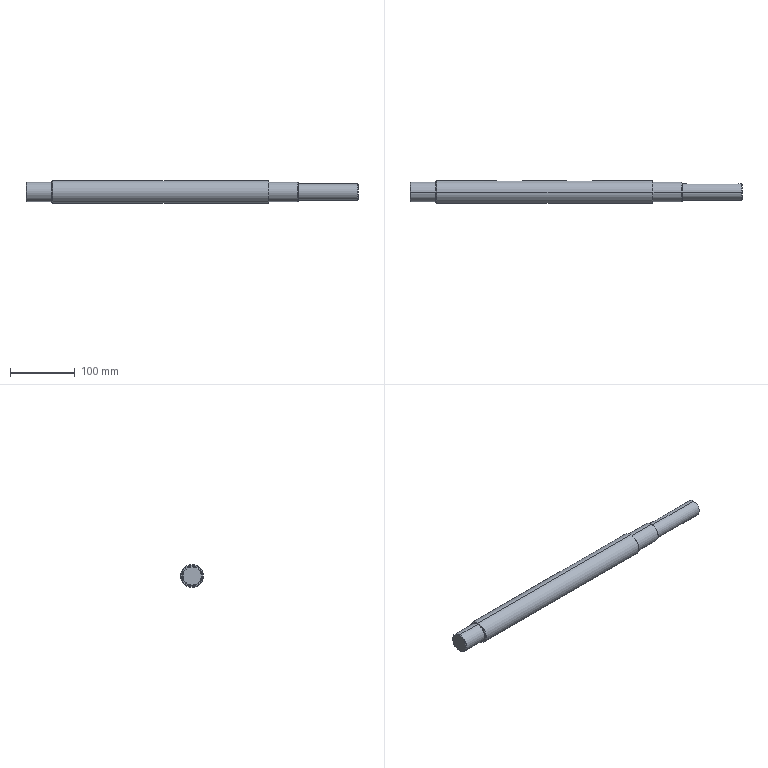Part | SolidWorks | features ICE 2, Chamfer 1, HoleWzd 1, Revolution 1 | 1 solid | 46 faces | box 511 x 35 x 35 mm | volume 419085 mm3 | cylinder 18 | cone 14 | plane 14 | commonest cylinder face diameters 5 x4 10 x4 30 x4 8 x2 25 x2 35 x2
STEP:
#1=CARTESIAN_POINT('',(284.,0.,-3.5));
#2=VERTEX_POINT('',#1);
#3=CARTESIAN_POINT('',(284.,0.,-8.5));
#4=VERTEX_POINT('',#3);
#5=CARTESIAN_POINT('',(284.,0.,-6.));
#6=DIRECTION('',(1.,0.,0.));
#7=DIRECTION('',(0.,0.,-1.));
#8=AXIS2_PLACEMENT_3D('',#5,#6,#7);
#9=CIRCLE('',#8,2.5);
#10=EDGE_CURVE('',#2,#4,#9,.T.);
#11=ORIENTED_EDGE('',*,*,#10,.F.);
#12=CARTESIAN_POINT('',(304.,0.,-3.5));
#13=VERTEX_POINT('',#12);
#14=CARTESIAN_POINT('',(304.,0.,-3.5));
#15=DIRECTION('',(1.,0.,0.));
#16=VECTOR('',#15,1000.);
#17=LINE('',#14,#16);
#18=EDGE_CURVE('',#2,#13,#17,.T.);
#19=ORIENTED_EDGE('',*,*,#18,.T.);
#20=CARTESIAN_POINT('',(304.,0.,-8.5));
#21=VERTEX_POINT('',#20);
#22=CARTESIAN_POINT('',(304.,0.,-6.));
#23=DIRECTION('',(1.,0.,0.));
#24=DIRECTION('',(0.,0.,-1.));
#25=AXIS2_PLACEMENT_3D('',#22,#23,#24);
#26=CIRCLE('',#25,2.5);
#27=EDGE_CURVE('',#13,#21,#26,.T.);
#28=ORIENTED_EDGE('',*,*,#27,.T.);
#29=CARTESIAN_POINT('',(304.,0.,-8.5));
#30=DIRECTION('',(1.,0.,0.));
#31=VECTOR('',#30,1000.);
#32=LINE('',#29,#31);
#33=EDGE_CURVE('',#4,#21,#32,.T.);
#34=ORIENTED_EDGE('',*,*,#33,.F.);
#35=EDGE_LOOP('',(#11,#19,#28,#34));
#36=FACE_OUTER_BOUND('',#35,.T.);
#37=CARTESIAN_POINT('',(304.,0.,-6.));
#38=DIRECTION('',(1.,0.,0.));
#39=DIRECTION('',(0.,0.,-1.));
#40=AXIS2_PLACEMENT_3D('',#37,#38,#39);
#41=CYLINDRICAL_SURFACE('',#40,2.5);
#42=ADVANCED_FACE('',(#36),#41,.F.);
#43=CARTESIAN_POINT('',(282.498,0.,-6.));
#44=VERTEX_POINT('',#43);
#45=CARTESIAN_POINT('',(284.,0.,-8.5));
#46=DIRECTION('',(0.515,0.,-0.8572));
#47=VECTOR('',#46,1000.);
#48=LINE('',#45,#47);
#49=EDGE_CURVE('',#44,#4,#48,.T.);
#50=ORIENTED_EDGE('',*,*,#49,.F.);
#51=CARTESIAN_POINT('',(284.,0.,-3.5));
#52=DIRECTION('',(0.515,0.,0.8572));
#53=VECTOR('',#52,1000.);
#54=LINE('',#51,#53);
#55=EDGE_CURVE('',#44,#2,#54,.T.);
#56=ORIENTED_EDGE('',*,*,#55,.T.);
#57=ORIENTED_EDGE('',*,*,#10,.T.);
#58=EDGE_LOOP('',(#50,#56,#57));
#59=FACE_OUTER_BOUND('',#58,.T.);
#60=CARTESIAN_POINT('',(284.,0.,-6.));
#61=DIRECTION('',(1.,0.,0.));
#62=DIRECTION('',(0.,0.,-1.));
#63=AXIS2_PLACEMENT_3D('',#60,#61,#62);
#64=CONICAL_SURFACE('',#63,2.5,1.03);
#65=ADVANCED_FACE('',(#59),#64,.F.);
#66=CARTESIAN_POINT('',(284.,0.,8.5));
#67=VERTEX_POINT('',#66);
#68=CARTESIAN_POINT('',(284.,0.,3.5));
#69=VERTEX_POINT('',#68);
#70=CARTESIAN_POINT('',(284.,0.,6.));
#71=DIRECTION('',(1.,0.,0.));
#72=DIRECTION('',(0.,0.,-1.));
#73=AXIS2_PLACEMENT_3D('',#70,#71,#72);
#74=CIRCLE('',#73,2.5);
#75=EDGE_CURVE('',#67,#69,#74,.T.);
#76=ORIENTED_EDGE('',*,*,#75,.F.);
#77=CARTESIAN_POINT('',(304.,0.,8.5));
#78=VERTEX_POINT('',#77);
#79=CARTESIAN_POINT('',(304.,0.,8.5));
#80=DIRECTION('',(1.,0.,0.));
#81=VECTOR('',#80,1000.);
#82=LINE('',#79,#81);
#83=EDGE_CURVE('',#67,#78,#82,.T.);
#84=ORIENTED_EDGE('',*,*,#83,.T.);
#85=CARTESIAN_POINT('',(304.,0.,3.5));
#86=VERTEX_POINT('',#85);
#87=CARTESIAN_POINT('',(304.,0.,6.));
#88=DIRECTION('',(1.,0.,0.));
#89=DIRECTION('',(0.,0.,-1.));
#90=AXIS2_PLACEMENT_3D('',#87,#88,#89);
#91=CIRCLE('',#90,2.5);
#92=EDGE_CURVE('',#78,#86,#91,.T.);
#93=ORIENTED_EDGE('',*,*,#92,.T.);
#94=CARTESIAN_POINT('',(304.,0.,3.5));
#95=DIRECTION('',(1.,0.,0.));
#96=VECTOR('',#95,1000.);
#97=LINE('',#94,#96);
#98=EDGE_CURVE('',#69,#86,#97,.T.);
#99=ORIENTED_EDGE('',*,*,#98,.F.);
#100=EDGE_LOOP('',(#76,#84,#93,#99));
#101=FACE_OUTER_BOUND('',#100,.T.);
#102=CARTESIAN_POINT('',(304.,0.,6.));
#103=DIRECTION('',(1.,0.,0.));
#104=DIRECTION('',(0.,0.,-1.));
#105=AXIS2_PLACEMENT_3D('',#102,#103,#104);
#106=CYLINDRICAL_SURFACE('',#105,2.5);
#107=ADVANCED_FACE('',(#101),#106,.F.);
#108=CARTESIAN_POINT('',(282.498,0.,6.));
#109=VERTEX_POINT('',#108);
#110=CARTESIAN_POINT('',(284.,0.,3.5));
#111=DIRECTION('',(0.515,0.,-0.8572));
#112=VECTOR('',#111,1000.);
#113=LINE('',#110,#112);
#114=EDGE_CURVE('',#109,#69,#113,.T.);
#115=ORIENTED_EDGE('',*,*,#114,.F.);
#116=CARTESIAN_POINT('',(284.,0.,8.5));
#117=DIRECTION('',(0.515,0.,0.8572));
#118=VECTOR('',#117,1000.);
#119=LINE('',#116,#118);
#120=EDGE_CURVE('',#109,#67,#119,.T.);
#121=ORIENTED_EDGE('',*,*,#120,.T.);
#122=ORIENTED_EDGE('',*,*,#75,.T.);
#123=EDGE_LOOP('',(#115,#121,#122));
#124=FACE_OUTER_BOUND('',#123,.T.);
#125=CARTESIAN_POINT('',(284.,0.,6.));
#126=DIRECTION('',(1.,0.,0.));
#127=DIRECTION('',(0.,0.,-1.));
#128=AXIS2_PLACEMENT_3D('',#125,#126,#127);
#129=CONICAL_SURFACE('',#128,2.5,1.03);
#130=ADVANCED_FACE('',(#124),#129,.F.);
#131=CARTESIAN_POINT('',(-207.,0.,14.));
#132=VERTEX_POINT('',#131);
#133=CARTESIAN_POINT('',(-207.,0.,-14.));
#134=VERTEX_POINT('',#133);
#135=CARTESIAN_POINT('',(-207.,0.,0.));
#136=DIRECTION('',(-1.,0.,0.));
#137=DIRECTION('',(0.,0.,1.));
#138=AXIS2_PLACEMENT_3D('',#135,#136,#137);
#139=CIRCLE('',#138,14.);
#140=EDGE_CURVE('',#132,#134,#139,.T.);
#141=ORIENTED_EDGE('',*,*,#140,.F.);
#142=CARTESIAN_POINT('',(-206.,0.,15.));
#143=VERTEX_POINT('',#142);
#144=CARTESIAN_POINT('',(-206.,0.,15.));
#145=DIRECTION('',(0.7071,0.,0.7071));
#146=VECTOR('',#145,1000.);
#147=LINE('',#144,#146);
#148=EDGE_CURVE('',#132,#143,#147,.T.);
#149=ORIENTED_EDGE('',*,*,#148,.T.);
#150=CARTESIAN_POINT('',(-206.,0.,-15.));
#151=VERTEX_POINT('',#150);
#152=CARTESIAN_POINT('',(-206.,0.,0.));
#153=DIRECTION('',(1.,0.,0.));
#154=DIRECTION('',(0.,0.,1.));
#155=AXIS2_PLACEMENT_3D('',#152,#153,#154);
#156=CIRCLE('',#155,15.);
#157=EDGE_CURVE('',#151,#143,#156,.T.);
#158=ORIENTED_EDGE('',*,*,#157,.F.);
#159=CARTESIAN_POINT('',(-206.,0.,-15.));
#160=DIRECTION('',(0.7071,0.,-0.7071));
#161=VECTOR('',#160,1000.);
#162=LINE('',#159,#161);
#163=EDGE_CURVE('',#134,#151,#162,.T.);
#164=ORIENTED_EDGE('',*,*,#163,.F.);
#165=EDGE_LOOP('',(#141,#149,#158,#164));
#166=FACE_OUTER_BOUND('',#165,.T.);
#167=CARTESIAN_POINT('',(-206.,0.,0.));
#168=DIRECTION('',(1.,0.,0.));
#169=DIRECTION('',(0.,0.,-1.));
#170=AXIS2_PLACEMENT_3D('',#167,#168,#169);
#171=CONICAL_SURFACE('',#170,15.,0.7854);
#172=ADVANCED_FACE('',(#166),#171,.T.);
#173=CARTESIAN_POINT('',(167.,0.,-16.5));
#174=VERTEX_POINT('',#173);
#175=CARTESIAN_POINT('',(167.,0.,16.5));
#176=VERTEX_POINT('',#175);
#177=CARTESIAN_POINT('',(167.,0.,0.));
#178=DIRECTION('',(1.,0.,0.));
#179=DIRECTION('',(0.,0.,-1.));
#180=AXIS2_PLACEMENT_3D('',#177,#178,#179);
#181=CIRCLE('',#180,16.5);
#182=EDGE_CURVE('',#174,#176,#181,.T.);
#183=ORIENTED_EDGE('',*,*,#182,.F.);
#184=CARTESIAN_POINT('',(166.,0.,-17.5));
#185=VERTEX_POINT('',#184);
#186=CARTESIAN_POINT('',(167.,0.,-16.5));
#187=DIRECTION('',(-0.7071,0.,-0.7071));
#188=VECTOR('',#187,1000.);
#189=LINE('',#186,#188);
#190=EDGE_CURVE('',#174,#185,#189,.T.);
#191=ORIENTED_EDGE('',*,*,#190,.T.);
#192=CARTESIAN_POINT('',(166.,0.,17.5));
#193=VERTEX_POINT('',#192);
#194=CARTESIAN_POINT('',(166.,0.,0.));
#195=DIRECTION('',(-1.,0.,0.));
#196=DIRECTION('',(0.,0.,-1.));
#197=AXIS2_PLACEMENT_3D('',#194,#195,#196);
#198=CIRCLE('',#197,17.5);
#199=EDGE_CURVE('',#193,#185,#198,.T.);
#200=ORIENTED_EDGE('',*,*,#199,.F.);
#201=CARTESIAN_POINT('',(167.,0.,16.5));
#202=DIRECTION('',(-0.7071,0.,0.7071));
#203=VECTOR('',#202,1000.);
#204=LINE('',#201,#203);
#205=EDGE_CURVE('',#176,#193,#204,.T.);
#206=ORIENTED_EDGE('',*,*,#205,.F.);
#207=EDGE_LOOP('',(#183,#191,#200,#206));
#208=FACE_OUTER_BOUND('',#207,.T.);
#209=CARTESIAN_POINT('',(167.,0.,0.));
#210=DIRECTION('',(-1.,0.,0.));
#211=DIRECTION('',(0.,0.,1.));
#212=AXIS2_PLACEMENT_3D('',#209,#210,#211);
#213=CONICAL_SURFACE('',#212,16.5,0.7854);
#214=ADVANCED_FACE('',(#208),#213,.T.);
#215=CARTESIAN_POINT('',(212.,0.,-14.));
#216=VERTEX_POINT('',#215);
#217=CARTESIAN_POINT('',(212.,0.,14.));
#218=VERTEX_POINT('',#217);
#219=CARTESIAN_POINT('',(212.,0.,0.));
#220=DIRECTION('',(1.,0.,0.));
#221=DIRECTION('',(0.,0.,-1.));
#222=AXIS2_PLACEMENT_3D('',#219,#220,#221);
#223=CIRCLE('',#222,14.);
#224=EDGE_CURVE('',#216,#218,#223,.T.);
#225=ORIENTED_EDGE('',*,*,#224,.F.);
#226=CARTESIAN_POINT('',(211.,0.,-15.));
#227=VERTEX_POINT('',#226);
#228=CARTESIAN_POINT('',(212.,0.,-14.));
#229=DIRECTION('',(-0.7071,0.,-0.7071));
#230=VECTOR('',#229,1000.);
#231=LINE('',#228,#230);
#232=EDGE_CURVE('',#216,#227,#231,.T.);
#233=ORIENTED_EDGE('',*,*,#232,.T.);
#234=CARTESIAN_POINT('',(211.,0.,15.));
#235=VERTEX_POINT('',#234);
#236=CARTESIAN_POINT('',(211.,0.,0.));
#237=DIRECTION('',(-1.,0.,0.));
#238=DIRECTION('',(0.,0.,-1.));
#239=AXIS2_PLACEMENT_3D('',#236,#237,#238);
#240=CIRCLE('',#239,15.);
#241=EDGE_CURVE('',#235,#227,#240,.T.);
#242=ORIENTED_EDGE('',*,*,#241,.F.);
#243=CARTESIAN_POINT('',(212.,0.,14.));
#244=DIRECTION('',(-0.7071,0.,0.7071));
#245=VECTOR('',#244,1000.);
#246=LINE('',#243,#245);
#247=EDGE_CURVE('',#218,#235,#246,.T.);
#248=ORIENTED_EDGE('',*,*,#247,.F.);
#249=EDGE_LOOP('',(#225,#233,#242,#248));
#250=FACE_OUTER_BOUND('',#249,.T.);
#251=CARTESIAN_POINT('',(212.,0.,0.));
#252=DIRECTION('',(-1.,0.,0.));
#253=DIRECTION('',(0.,0.,1.));
#254=AXIS2_PLACEMENT_3D('',#251,#252,#253);
#255=CONICAL_SURFACE('',#254,14.,0.7854);
#256=ADVANCED_FACE('',(#250),#255,.T.);
#257=CARTESIAN_POINT('',(304.,0.,-11.5));
#258=VERTEX_POINT('',#257);
#259=CARTESIAN_POINT('',(304.,0.,11.5));
#260=VERTEX_POINT('',#259);
#261=CARTESIAN_POINT('',(304.,0.,0.));
#262=DIRECTION('',(1.,0.,0.));
#263=DIRECTION('',(0.,0.,-1.));
#264=AXIS2_PLACEMENT_3D('',#261,#262,#263);
#265=CIRCLE('',#264,11.5);
#266=EDGE_CURVE('',#258,#260,#265,.T.);
#267=ORIENTED_EDGE('',*,*,#266,.F.);
#268=CARTESIAN_POINT('',(303.,0.,-12.5));
#269=VERTEX_POINT('',#268);
#270=CARTESIAN_POINT('',(304.,0.,-11.5));
#271=DIRECTION('',(-0.7071,0.,-0.7071));
#272=VECTOR('',#271,1000.);
#273=LINE('',#270,#272);
#274=EDGE_CURVE('',#258,#269,#273,.T.);
#275=ORIENTED_EDGE('',*,*,#274,.T.);
#276=CARTESIAN_POINT('',(303.,0.,12.5));
#277=VERTEX_POINT('',#276);
#278=CARTESIAN_POINT('',(303.,0.,0.));
#279=DIRECTION('',(-1.,0.,0.));
#280=DIRECTION('',(0.,0.,-1.));
#281=AXIS2_PLACEMENT_3D('',#278,#279,#280);
#282=CIRCLE('',#281,12.5);
#283=EDGE_CURVE('',#277,#269,#282,.T.);
#284=ORIENTED_EDGE('',*,*,#283,.F.);
#285=CARTESIAN_POINT('',(304.,0.,11.5));
#286=DIRECTION('',(-0.7071,0.,0.7071));
#287=VECTOR('',#286,1000.);
#288=LINE('',#285,#287);
#289=EDGE_CURVE('',#260,#277,#288,.T.);
#290=ORIENTED_EDGE('',*,*,#289,.F.);
#291=EDGE_LOOP('',(#267,#275,#284,#290));
#292=FACE_OUTER_BOUND('',#291,.T.);
#293=CARTESIAN_POINT('',(304.,0.,0.));
#294=DIRECTION('',(-1.,0.,0.));
#295=DIRECTION('',(0.,0.,1.));
#296=AXIS2_PLACEMENT_3D('',#293,#294,#295);
#297=CONICAL_SURFACE('',#296,11.5,0.7854);
#298=ADVANCED_FACE('',(#292),#297,.T.);
#299=CARTESIAN_POINT('',(-167.,0.,16.5));
#300=VERTEX_POINT('',#299);
#301=CARTESIAN_POINT('',(-167.,0.,-16.5));
#302=VERTEX_POINT('',#301);
#303=CARTESIAN_POINT('',(-167.,0.,0.));
#304=DIRECTION('',(-1.,0.,0.));
#305=DIRECTION('',(0.,0.,1.));
#306=AXIS2_PLACEMENT_3D('',#303,#304,#305);
#307=CIRCLE('',#306,16.5);
#308=EDGE_CURVE('',#300,#302,#307,.T.);
#309=ORIENTED_EDGE('',*,*,#308,.F.);
#310=CARTESIAN_POINT('',(-166.,0.,17.5));
#311=VERTEX_POINT('',#310);
#312=CARTESIAN_POINT('',(-166.,0.,17.5));
#313=DIRECTION('',(0.7071,0.,0.7071));
#314=VECTOR('',#313,1000.);
#315=LINE('',#312,#314);
#316=EDGE_CURVE('',#300,#311,#315,.T.);
#317=ORIENTED_EDGE('',*,*,#316,.T.);
#318=CARTESIAN_POINT('',(-166.,0.,-17.5));
#319=VERTEX_POINT('',#318);
#320=CARTESIAN_POINT('',(-166.,0.,0.));
#321=DIRECTION('',(1.,0.,0.));
#322=DIRECTION('',(0.,0.,1.));
#323=AXIS2_PLACEMENT_3D('',#320,#321,#322);
#324=CIRCLE('',#323,17.5);
#325=EDGE_CURVE('',#319,#311,#324,.T.);
#326=ORIENTED_EDGE('',*,*,#325,.F.);
#327=CARTESIAN_POINT('',(-166.,0.,-17.5));
#328=DIRECTION('',(0.7071,0.,-0.7071));
#329=VECTOR('',#328,1000.);
#330=LINE('',#327,#329);
#331=EDGE_CURVE('',#302,#319,#330,.T.);
#332=ORIENTED_EDGE('',*,*,#331,.F.);
#333=EDGE_LOOP('',(#309,#317,#326,#332));
#334=FACE_OUTER_BOUND('',#333,.T.);
#335=CARTESIAN_POINT('',(-166.,0.,0.));
#336=DIRECTION('',(1.,0.,0.));
#337=DIRECTION('',(0.,0.,-1.));
#338=AXIS2_PLACEMENT_3D('',#335,#336,#337);
#339=CONICAL_SURFACE('',#338,17.5,0.7854);
#340=ADVANCED_FACE('',(#334),#339,.T.);
#341=CARTESIAN_POINT('',(167.,0.,-15.));
#342=VERTEX_POINT('',#341);
#343=CARTESIAN_POINT('',(167.,0.,15.));
#344=VERTEX_POINT('',#343);
#345=CARTESIAN_POINT('',(167.,0.,0.));
#346=DIRECTION('',(1.,0.,0.));
#347=DIRECTION('',(0.,0.,-1.));
#348=AXIS2_PLACEMENT_3D('',#345,#346,#347);
#349=CIRCLE('',#348,15.);
#350=EDGE_CURVE('',#342,#344,#349,.T.);
#351=ORIENTED_EDGE('',*,*,#350,.T.);
#352=CARTESIAN_POINT('',(0.,0.,15.));
#353=DIRECTION('',(1.,0.,0.));
#354=VECTOR('',#353,1000.);
#355=LINE('',#352,#354);
#356=EDGE_CURVE('',#344,#235,#355,.T.);
#357=ORIENTED_EDGE('',*,*,#356,.T.);
#358=ORIENTED_EDGE('',*,*,#241,.T.);
#359=CARTESIAN_POINT('',(0.,0.,-15.));
#360=DIRECTION('',(1.,0.,0.));
#361=VECTOR('',#360,1000.);
#362=LINE('',#359,#361);
#363=EDGE_CURVE('',#342,#227,#362,.T.);
#364=ORIENTED_EDGE('',*,*,#363,.F.);
#365=EDGE_LOOP('',(#351,#357,#358,#364));
#366=FACE_OUTER_BOUND('',#365,.T.);
#367=CARTESIAN_POINT('',(0.,0.,0.));
#368=DIRECTION('',(1.,0.,0.));
#369=DIRECTION('',(0.,0.,-1.));
#370=AXIS2_PLACEMENT_3D('',#367,#368,#369);
#371=CYLINDRICAL_SURFACE('',#370,15.);
#372=ADVANCED_FACE('',(#366),#371,.T.);
#373=CARTESIAN_POINT('',(295.,11.843,4.));
#374=VERTEX_POINT('',#373);
#375=CARTESIAN_POINT('',(295.,11.843,-4.));
#376=VERTEX_POINT('',#375);
#377=CARTESIAN_POINT('',(295.,11.843,4.));
#378=CARTESIAN_POINT('',(295.266,11.843,4.));
#379=CARTESIAN_POINT('',(295.527,11.852,3.974));
#380=CARTESIAN_POINT('',(296.041,11.886,3.871));
#381=CARTESIAN_POINT('',(296.296,11.911,3.793));
#382=CARTESIAN_POINT('',(296.779,11.973,3.592));
#383=CARTESIAN_POINT('',(297.008,12.01,3.469));
#384=CARTESIAN_POINT('',(297.441,12.09,3.179));
#385=CARTESIAN_POINT('',(297.645,12.133,3.012));
#386=CARTESIAN_POINT('',(298.011,12.218,2.646));
#387=CARTESIAN_POINT('',(298.176,12.26,2.445));
#388=CARTESIAN_POINT('',(298.469,12.34,2.009));
#389=CARTESIAN_POINT('',(298.592,12.375,1.779));
#390=CARTESIAN_POINT('',(298.792,12.435,1.299));
#391=CARTESIAN_POINT('',(298.87,12.459,1.045));
#392=CARTESIAN_POINT('',(298.974,12.492,0.5276));
#393=CARTESIAN_POINT('',(299.,12.5,0.2669));
#394=CARTESIAN_POINT('',(299.,12.5,-0.2587));
#395=CARTESIAN_POINT('',(298.974,12.492,-0.5256));
#396=CARTESIAN_POINT('',(298.871,12.459,-1.04));
#397=CARTESIAN_POINT('',(298.795,12.436,-1.29));
#398=CARTESIAN_POINT('',(298.593,12.375,-1.777));
#399=CARTESIAN_POINT('',(298.469,12.34,-2.008));
#400=CARTESIAN_POINT('',(298.18,12.262,-2.44));
#401=CARTESIAN_POINT('',(298.013,12.219,-2.643));
#402=CARTESIAN_POINT('',(297.645,12.133,-3.012));
#403=CARTESIAN_POINT('',(297.445,12.091,-3.176));
#404=CARTESIAN_POINT('',(297.013,12.011,-3.466));
#405=CARTESIAN_POINT('',(296.78,11.973,-3.592));
#406=CARTESIAN_POINT('',(296.298,11.911,-3.792));
#407=CARTESIAN_POINT('',(296.049,11.886,-3.869));
#408=CARTESIAN_POINT('',(295.532,11.852,-3.973));
#409=CARTESIAN_POINT('',(295.266,11.843,-4.));
#410=CARTESIAN_POINT('',(295.,11.843,-4.));
#411=B_SPLINE_CURVE_WITH_KNOTS('',3,(#377,#378,#379,#380,#381,#382,#383,#384,#385,#386,#387,#388,#389,#390,#391,#392,#393,#394,#395,#396,#397,#398,#399,#400,#401,#402,#403,#404,#405,#406,#407,#408,#409,#410),.UNSPECIFIED.,.F.,.F.,(4,2,2,2,2,2,2,2,2,2,2,2,2,2,2,2,4),(0.,0.0007865,0.001573,0.00236,0.003146,0.003933,0.004719,0.005506,0.006292,0.007079,0.007865,0.008652,0.009438,0.01022,0.01101,0.0118,0.01258),.UNSPECIFIED.);
#412=EDGE_CURVE('',#374,#376,#411,.T.);
#413=ORIENTED_EDGE('',*,*,#412,.F.);
#414=CARTESIAN_POINT('',(223.,11.843,4.));
#415=VERTEX_POINT('',#414);
#416=CARTESIAN_POINT('',(0.,11.843,4.));
#417=DIRECTION('',(1.,0.,0.));
#418=VECTOR('',#417,1000.);
#419=LINE('',#416,#418);
#420=EDGE_CURVE('',#415,#374,#419,.T.);
#421=ORIENTED_EDGE('',*,*,#420,.F.);
#422=CARTESIAN_POINT('',(223.,11.843,-4.));
#423=VERTEX_POINT('',#422);
#424=CARTESIAN_POINT('',(223.,11.843,-4.));
#425=CARTESIAN_POINT('',(222.734,11.843,-4.));
#426=CARTESIAN_POINT('',(222.473,11.852,-3.974));
#427=CARTESIAN_POINT('',(221.959,11.886,-3.871));
#428=CARTESIAN_POINT('',(221.704,11.911,-3.793));
#429=CARTESIAN_POINT('',(221.221,11.973,-3.592));
#430=CARTESIAN_POINT('',(220.992,12.01,-3.469));
#431=CARTESIAN_POINT('',(220.559,12.09,-3.179));
#432=CARTESIAN_POINT('',(220.355,12.133,-3.012));
#433=CARTESIAN_POINT('',(219.989,12.218,-2.646));
#434=CARTESIAN_POINT('',(219.824,12.26,-2.445));
#435=CARTESIAN_POINT('',(219.531,12.34,-2.009));
#436=CARTESIAN_POINT('',(219.408,12.375,-1.779));
#437=CARTESIAN_POINT('',(219.208,12.435,-1.299));
#438=CARTESIAN_POINT('',(219.13,12.459,-1.045));
#439=CARTESIAN_POINT('',(219.026,12.492,-0.5276));
#440=CARTESIAN_POINT('',(219.,12.5,-0.2669));
#441=CARTESIAN_POINT('',(219.,12.5,0.2587));
#442=CARTESIAN_POINT('',(219.026,12.492,0.5256));
#443=CARTESIAN_POINT('',(219.129,12.459,1.04));
#444=CARTESIAN_POINT('',(219.205,12.436,1.29));
#445=CARTESIAN_POINT('',(219.407,12.375,1.777));
#446=CARTESIAN_POINT('',(219.531,12.34,2.008));
#447=CARTESIAN_POINT('',(219.82,12.262,2.44));
#448=CARTESIAN_POINT('',(219.987,12.219,2.643));
#449=CARTESIAN_POINT('',(220.355,12.133,3.012));
#450=CARTESIAN_POINT('',(220.555,12.091,3.176));
#451=CARTESIAN_POINT('',(220.987,12.011,3.466));
#452=CARTESIAN_POINT('',(221.22,11.973,3.592));
#453=CARTESIAN_POINT('',(221.702,11.911,3.792));
#454=CARTESIAN_POINT('',(221.951,11.886,3.869));
#455=CARTESIAN_POINT('',(222.468,11.852,3.973));
#456=CARTESIAN_POINT('',(222.734,11.843,4.));
#457=CARTESIAN_POINT('',(223.,11.843,4.));
#458=B_SPLINE_CURVE_WITH_KNOTS('',3,(#424,#425,#426,#427,#428,#429,#430,#431,#432,#433,#434,#435,#436,#437,#438,#439,#440,#441,#442,#443,#444,#445,#446,#447,#448,#449,#450,#451,#452,#453,#454,#455,#456,#457),.UNSPECIFIED.,.F.,.F.,(4,2,2,2,2,2,2,2,2,2,2,2,2,2,2,2,4),(0.,0.0007865,0.001573,0.00236,0.003146,0.003933,0.004719,0.005506,0.006292,0.007079,0.007865,0.008652,0.009438,0.01022,0.01101,0.0118,0.01258),.UNSPECIFIED.);
#459=EDGE_CURVE('',#423,#415,#458,.T.);
#460=ORIENTED_EDGE('',*,*,#459,.F.);
#461=CARTESIAN_POINT('',(0.,11.843,-4.));
#462=DIRECTION('',(-1.,0.,0.));
#463=VECTOR('',#462,1000.);
#464=LINE('',#461,#463);
#465=EDGE_CURVE('',#376,#423,#464,.T.);
#466=ORIENTED_EDGE('',*,*,#465,.F.);
#467=EDGE_LOOP('',(#413,#421,#460,#466));
#468=FACE_BOUND('',#467,.T.);
#469=CARTESIAN_POINT('',(212.,0.,-12.5));
#470=VERTEX_POINT('',#469);
#471=CARTESIAN_POINT('',(212.,0.,12.5));
#472=VERTEX_POINT('',#471);
#473=CARTESIAN_POINT('',(212.,0.,0.));
#474=DIRECTION('',(1.,0.,0.));
#475=DIRECTION('',(0.,0.,-1.));
#476=AXIS2_PLACEMENT_3D('',#473,#474,#475);
#477=CIRCLE('',#476,12.5);
#478=EDGE_CURVE('',#470,#472,#477,.T.);
#479=ORIENTED_EDGE('',*,*,#478,.T.);
#480=CARTESIAN_POINT('',(0.,0.,12.5));
#481=DIRECTION('',(1.,0.,0.));
#482=VECTOR('',#481,1000.);
#483=LINE('',#480,#482);
#484=EDGE_CURVE('',#472,#277,#483,.T.);
#485=ORIENTED_EDGE('',*,*,#484,.T.);
#486=ORIENTED_EDGE('',*,*,#283,.T.);
#487=CARTESIAN_POINT('',(0.,0.,-12.5));
#488=DIRECTION('',(1.,0.,0.));
#489=VECTOR('',#488,1000.);
#490=LINE('',#487,#489);
#491=EDGE_CURVE('',#470,#269,#490,.T.);
#492=ORIENTED_EDGE('',*,*,#491,.F.);
#493=EDGE_LOOP('',(#479,#485,#486,#492));
#494=FACE_OUTER_BOUND('',#493,.T.);
#495=CARTESIAN_POINT('',(0.,0.,0.));
#496=DIRECTION('',(1.,0.,0.));
#497=DIRECTION('',(0.,0.,-1.));
#498=AXIS2_PLACEMENT_3D('',#495,#496,#497);
#499=CYLINDRICAL_SURFACE('',#498,12.5);
#500=ADVANCED_FACE('',(#468,#494),#499,.T.);
#501=ORIENTED_EDGE('',*,*,#157,.T.);
#502=CARTESIAN_POINT('',(-167.,0.,15.));
#503=VERTEX_POINT('',#502);
#504=CARTESIAN_POINT('',(0.,0.,15.));
#505=DIRECTION('',(1.,0.,0.));
#506=VECTOR('',#505,1000.);
#507=LINE('',#504,#506);
#508=EDGE_CURVE('',#143,#503,#507,.T.);
#509=ORIENTED_EDGE('',*,*,#508,.T.);
#510=CARTESIAN_POINT('',(-167.,0.,-15.));
#511=VERTEX_POINT('',#510);
#512=CARTESIAN_POINT('',(-167.,0.,0.));
#513=DIRECTION('',(1.,0.,0.));
#514=DIRECTION('',(0.,0.,-1.));
#515=AXIS2_PLACEMENT_3D('',#512,#513,#514);
#516=CIRCLE('',#515,15.);
#517=EDGE_CURVE('',#511,#503,#516,.T.);
#518=ORIENTED_EDGE('',*,*,#517,.F.);
#519=CARTESIAN_POINT('',(0.,0.,-15.));
#520=DIRECTION('',(1.,0.,0.));
#521=VECTOR('',#520,1000.);
#522=LINE('',#519,#521);
#523=EDGE_CURVE('',#151,#511,#522,.T.);
#524=ORIENTED_EDGE('',*,*,#523,.F.);
#525=EDGE_LOOP('',(#501,#509,#518,#524));
#526=FACE_OUTER_BOUND('',#525,.T.);
#527=CARTESIAN_POINT('',(0.,0.,0.));
#528=DIRECTION('',(1.,0.,0.));
#529=DIRECTION('',(0.,0.,-1.));
#530=AXIS2_PLACEMENT_3D('',#527,#528,#529);
#531=CYLINDRICAL_SURFACE('',#530,15.);
#532=ADVANCED_FACE('',(#526),#531,.T.);
#533=CARTESIAN_POINT('',(-71.5,16.771,-5.));
#534=VERTEX_POINT('',#533);
#535=CARTESIAN_POINT('',(-71.5,16.771,5.));
#536=VERTEX_POINT('',#535);
#537=CARTESIAN_POINT('',(-71.5,16.771,-5.));
#538=CARTESIAN_POINT('',(-71.832,16.771,-5.));
#539=CARTESIAN_POINT('',(-72.158,16.78,-4.967));
#540=CARTESIAN_POINT('',(-72.8,16.818,-4.839));
#541=CARTESIAN_POINT('',(-73.118,16.846,-4.742));
#542=CARTESIAN_POINT('',(-73.722,16.914,-4.491));
#543=CARTESIAN_POINT('',(-74.009,16.955,-4.337));
#544=CARTESIAN_POINT('',(-74.551,17.044,-3.975));
#545=CARTESIAN_POINT('',(-74.806,17.092,-3.765));
#546=CARTESIAN_POINT('',(-75.265,17.186,-3.306));
#547=CARTESIAN_POINT('',(-75.471,17.233,-3.056));
#548=CARTESIAN_POINT('',(-75.837,17.321,-2.51));
#549=CARTESIAN_POINT('',(-75.991,17.361,-2.222));
#550=CARTESIAN_POINT('',(-76.179,17.411,-1.771));
#551=CARTESIAN_POINT('',(-76.234,17.426,-1.618));
#552=CARTESIAN_POINT('',(-76.33,17.452,-1.304));
#553=CARTESIAN_POINT('',(-76.37,17.463,-1.143));
#554=CARTESIAN_POINT('',(-76.467,17.491,-0.6583));
#555=CARTESIAN_POINT('',(-76.5,17.5,-0.3328));
#556=CARTESIAN_POINT('',(-76.5,17.5,0.3232));
#557=CARTESIAN_POINT('',(-76.468,17.491,0.6564));
#558=CARTESIAN_POINT('',(-76.339,17.455,1.299));
#559=CARTESIAN_POINT('',(-76.245,17.428,1.612));
#560=CARTESIAN_POINT('',(-75.993,17.361,2.219));
#561=CARTESIAN_POINT('',(-75.837,17.321,2.509));
#562=CARTESIAN_POINT('',(-75.476,17.235,3.049));
#563=CARTESIAN_POINT('',(-75.268,17.187,3.303));
#564=CARTESIAN_POINT('',(-74.806,17.092,3.765));
#565=CARTESIAN_POINT('',(-74.555,17.045,3.971));
#566=CARTESIAN_POINT('',(-74.016,16.956,4.333));
#567=CARTESIAN_POINT('',(-73.723,16.915,4.49));
#568=CARTESIAN_POINT('',(-73.121,16.846,4.741));
#569=CARTESIAN_POINT('',(-72.809,16.818,4.837));
#570=CARTESIAN_POINT('',(-72.164,16.781,4.967));
#571=CARTESIAN_POINT('',(-71.832,16.771,5.));
#572=CARTESIAN_POINT('',(-71.5,16.771,5.));
#573=B_SPLINE_CURVE_WITH_KNOTS('',3,(#537,#538,#539,#540,#541,#542,#543,#544,#545,#546,#547,#548,#549,#550,#551,#552,#553,#554,#555,#556,#557,#558,#559,#560,#561,#562,#563,#564,#565,#566,#567,#568,#569,#570,#571,#572),.UNSPECIFIED.,.F.,.F.,(4,2,2,2,2,2,2,2,2,2,2,2,2,2,2,2,2,4),(0.,0.0009818,0.001964,0.002945,0.003927,0.004909,0.005891,0.006382,0.006873,0.007855,0.008836,0.009818,0.0108,0.01178,0.01276,0.01375,0.01473,0.01571),.UNSPECIFIED.);
#574=EDGE_CURVE('',#534,#536,#573,.T.);
#575=ORIENTED_EDGE('',*,*,#574,.F.);
#576=CARTESIAN_POINT('',(-36.5,16.771,-5.));
#577=VERTEX_POINT('',#576);
#578=CARTESIAN_POINT('',(0.,16.771,-5.));
#579=DIRECTION('',(-1.,0.,0.));
#580=VECTOR('',#579,1000.);
#581=LINE('',#578,#580);
#582=EDGE_CURVE('',#577,#534,#581,.T.);
#583=ORIENTED_EDGE('',*,*,#582,.F.);
#584=CARTESIAN_POINT('',(-36.5,16.771,5.));
#585=VERTEX_POINT('',#584);
#586=CARTESIAN_POINT('',(-36.5,16.771,5.));
#587=CARTESIAN_POINT('',(-36.168,16.771,5.));
#588=CARTESIAN_POINT('',(-35.841,16.78,4.967));
#589=CARTESIAN_POINT('',(-35.2,16.818,4.839));
#590=CARTESIAN_POINT('',(-34.882,16.846,4.742));
#591=CARTESIAN_POINT('',(-34.277,16.915,4.491));
#592=CARTESIAN_POINT('',(-33.99,16.955,4.337));
#593=CARTESIAN_POINT('',(-33.448,17.044,3.974));
#594=CARTESIAN_POINT('',(-33.193,17.092,3.764));
#595=CARTESIAN_POINT('',(-32.734,17.187,3.305));
#596=CARTESIAN_POINT('',(-32.528,17.234,3.055));
#597=CARTESIAN_POINT('',(-32.162,17.321,2.509));
#598=CARTESIAN_POINT('',(-32.008,17.361,2.22));
#599=CARTESIAN_POINT('',(-31.821,17.411,1.77));
#600=CARTESIAN_POINT('',(-31.765,17.426,1.616));
#601=CARTESIAN_POINT('',(-31.67,17.452,1.302));
#602=CARTESIAN_POINT('',(-31.629,17.464,1.141));
#603=CARTESIAN_POINT('',(-31.532,17.491,0.6559));
#604=CARTESIAN_POINT('',(-31.5,17.5,0.3302));
#605=CARTESIAN_POINT('',(-31.5,17.5,-0.326));
#606=CARTESIAN_POINT('',(-31.533,17.491,-0.6593));
#607=CARTESIAN_POINT('',(-31.661,17.454,-1.302));
#608=CARTESIAN_POINT('',(-31.756,17.428,-1.615));
#609=CARTESIAN_POINT('',(-32.009,17.361,-2.222));
#610=CARTESIAN_POINT('',(-32.165,17.321,-2.512));
#611=CARTESIAN_POINT('',(-32.526,17.234,-3.052));
#612=CARTESIAN_POINT('',(-32.735,17.186,-3.306));
#613=CARTESIAN_POINT('',(-33.197,17.091,-3.768));
#614=CARTESIAN_POINT('',(-33.448,17.044,-3.974));
#615=CARTESIAN_POINT('',(-33.988,16.955,-4.335));
#616=CARTESIAN_POINT('',(-34.281,16.914,-4.492));
#617=CARTESIAN_POINT('',(-34.884,16.846,-4.743));
#618=CARTESIAN_POINT('',(-35.196,16.818,-4.838));
#619=CARTESIAN_POINT('',(-35.679,16.79,-4.935));
#620=CARTESIAN_POINT('',(-35.844,16.783,-4.96));
#621=CARTESIAN_POINT('',(-36.172,16.773,-4.992));
#622=CARTESIAN_POINT('',(-36.336,16.771,-5.));
#623=CARTESIAN_POINT('',(-36.5,16.771,-5.));
#624=B_SPLINE_CURVE_WITH_KNOTS('',3,(#586,#587,#588,#589,#590,#591,#592,#593,#594,#595,#596,#597,#598,#599,#600,#601,#602,#603,#604,#605,#606,#607,#608,#609,#610,#611,#612,#613,#614,#615,#616,#617,#618,#619,#620,#621,#622,#623),.UNSPECIFIED.,.F.,.F.,(4,2,2,2,2,2,2,2,2,2,2,2,2,2,2,2,2,2,4),(0.,0.0009821,0.001964,0.002946,0.003929,0.004911,0.005893,0.006384,0.006875,0.007857,0.008839,0.009821,0.0108,0.01179,0.01277,0.01375,0.01473,0.01522,0.01571),.UNSPECIFIED.);
#625=EDGE_CURVE('',#585,#577,#624,.T.);
#626=ORIENTED_EDGE('',*,*,#625,.F.);
#627=CARTESIAN_POINT('',(0.,16.771,5.));
#628=DIRECTION('',(1.,0.,0.));
#629=VECTOR('',#628,1000.);
#630=LINE('',#627,#629);
#631=EDGE_CURVE('',#536,#585,#630,.T.);
#632=ORIENTED_EDGE('',*,*,#631,.F.);
#633=EDGE_LOOP('',(#575,#583,#626,#632));
#634=FACE_BOUND('',#633,.T.);
#635=CARTESIAN_POINT('',(71.5,16.771,5.));
#636=VERTEX_POINT('',#635);
#637=CARTESIAN_POINT('',(71.5,16.771,-5.));
#638=VERTEX_POINT('',#637);
#639=CARTESIAN_POINT('',(71.5,16.771,5.));
#640=CARTESIAN_POINT('',(71.832,16.771,5.));
#641=CARTESIAN_POINT('',(72.159,16.78,4.967));
#642=CARTESIAN_POINT('',(72.8,16.818,4.839));
#643=CARTESIAN_POINT('',(73.118,16.846,4.742));
#644=CARTESIAN_POINT('',(73.723,16.915,4.491));
#645=CARTESIAN_POINT('',(74.01,16.955,4.337));
#646=CARTESIAN_POINT('',(74.552,17.044,3.974));
#647=CARTESIAN_POINT('',(74.807,17.092,3.764));
#648=CARTESIAN_POINT('',(75.266,17.187,3.305));
#649=CARTESIAN_POINT('',(75.472,17.234,3.055));
#650=CARTESIAN_POINT('',(75.838,17.321,2.509));
#651=CARTESIAN_POINT('',(75.992,17.361,2.22));
#652=CARTESIAN_POINT('',(76.179,17.411,1.77));
#653=CARTESIAN_POINT('',(76.235,17.426,1.616));
#654=CARTESIAN_POINT('',(76.33,17.452,1.302));
#655=CARTESIAN_POINT('',(76.371,17.464,1.141));
#656=CARTESIAN_POINT('',(76.468,17.491,0.6559));
#657=CARTESIAN_POINT('',(76.5,17.5,0.3302));
#658=CARTESIAN_POINT('',(76.5,17.5,-0.326));
#659=CARTESIAN_POINT('',(76.467,17.491,-0.6593));
#660=CARTESIAN_POINT('',(76.339,17.454,-1.302));
#661=CARTESIAN_POINT('',(76.244,17.428,-1.615));
#662=CARTESIAN_POINT('',(75.991,17.361,-2.222));
#663=CARTESIAN_POINT('',(75.835,17.321,-2.512));
#664=CARTESIAN_POINT('',(75.474,17.234,-3.052));
#665=CARTESIAN_POINT('',(75.265,17.186,-3.306));
#666=CARTESIAN_POINT('',(74.803,17.091,-3.768));
#667=CARTESIAN_POINT('',(74.552,17.044,-3.974));
#668=CARTESIAN_POINT('',(74.012,16.955,-4.335));
#669=CARTESIAN_POINT('',(73.719,16.914,-4.492));
#670=CARTESIAN_POINT('',(73.116,16.846,-4.743));
#671=CARTESIAN_POINT('',(72.804,16.818,-4.838));
#672=CARTESIAN_POINT('',(72.321,16.79,-4.935));
#673=CARTESIAN_POINT('',(72.156,16.783,-4.96));
#674=CARTESIAN_POINT('',(71.828,16.773,-4.992));
#675=CARTESIAN_POINT('',(71.664,16.771,-5.));
#676=CARTESIAN_POINT('',(71.5,16.771,-5.));
#677=B_SPLINE_CURVE_WITH_KNOTS('',3,(#639,#640,#641,#642,#643,#644,#645,#646,#647,#648,#649,#650,#651,#652,#653,#654,#655,#656,#657,#658,#659,#660,#661,#662,#663,#664,#665,#666,#667,#668,#669,#670,#671,#672,#673,#674,#675,#676),.UNSPECIFIED.,.F.,.F.,(4,2,2,2,2,2,2,2,2,2,2,2,2,2,2,2,2,2,4),(0.,0.0009821,0.001964,0.002946,0.003929,0.004911,0.005893,0.006384,0.006875,0.007857,0.008839,0.009821,0.0108,0.01179,0.01277,0.01375,0.01473,0.01522,0.01571),.UNSPECIFIED.);
#678=EDGE_CURVE('',#636,#638,#677,.T.);
#679=ORIENTED_EDGE('',*,*,#678,.F.);
#680=CARTESIAN_POINT('',(36.5,16.771,5.));
#681=VERTEX_POINT('',#680);
#682=CARTESIAN_POINT('',(0.,16.771,5.));
#683=DIRECTION('',(1.,0.,0.));
#684=VECTOR('',#683,1000.);
#685=LINE('',#682,#684);
#686=EDGE_CURVE('',#681,#636,#685,.T.);
#687=ORIENTED_EDGE('',*,*,#686,.F.);
#688=CARTESIAN_POINT('',(36.5,16.771,-5.));
#689=VERTEX_POINT('',#688);
#690=CARTESIAN_POINT('',(36.5,16.771,-5.));
#691=CARTESIAN_POINT('',(36.168,16.771,-5.));
#692=CARTESIAN_POINT('',(35.842,16.78,-4.967));
#693=CARTESIAN_POINT('',(35.2,16.818,-4.839));
#694=CARTESIAN_POINT('',(34.882,16.846,-4.742));
#695=CARTESIAN_POINT('',(34.278,16.914,-4.491));
#696=CARTESIAN_POINT('',(33.991,16.955,-4.337));
#697=CARTESIAN_POINT('',(33.449,17.044,-3.975));
#698=CARTESIAN_POINT('',(33.194,17.092,-3.765));
#699=CARTESIAN_POINT('',(32.735,17.186,-3.306));
#700=CARTESIAN_POINT('',(32.529,17.233,-3.056));
#701=CARTESIAN_POINT('',(32.163,17.321,-2.51));
#702=CARTESIAN_POINT('',(32.009,17.361,-2.222));
#703=CARTESIAN_POINT('',(31.821,17.411,-1.771));
#704=CARTESIAN_POINT('',(31.766,17.426,-1.618));
#705=CARTESIAN_POINT('',(31.67,17.452,-1.304));
#706=CARTESIAN_POINT('',(31.63,17.463,-1.143));
#707=CARTESIAN_POINT('',(31.533,17.491,-0.6583));
#708=CARTESIAN_POINT('',(31.5,17.5,-0.3328));
#709=CARTESIAN_POINT('',(31.5,17.5,0.3232));
#710=CARTESIAN_POINT('',(31.532,17.491,0.6564));
#711=CARTESIAN_POINT('',(31.661,17.455,1.299));
#712=CARTESIAN_POINT('',(31.755,17.428,1.612));
#713=CARTESIAN_POINT('',(32.007,17.361,2.219));
#714=CARTESIAN_POINT('',(32.163,17.321,2.509));
#715=CARTESIAN_POINT('',(32.524,17.235,3.049));
#716=CARTESIAN_POINT('',(32.732,17.187,3.303));
#717=CARTESIAN_POINT('',(33.194,17.092,3.765));
#718=CARTESIAN_POINT('',(33.445,17.045,3.971));
#719=CARTESIAN_POINT('',(33.984,16.956,4.333));
#720=CARTESIAN_POINT('',(34.277,16.915,4.49));
#721=CARTESIAN_POINT('',(34.879,16.846,4.741));
#722=CARTESIAN_POINT('',(35.191,16.818,4.837));
#723=CARTESIAN_POINT('',(35.836,16.781,4.967));
#724=CARTESIAN_POINT('',(36.168,16.771,5.));
#725=CARTESIAN_POINT('',(36.5,16.771,5.));
#726=B_SPLINE_CURVE_WITH_KNOTS('',3,(#690,#691,#692,#693,#694,#695,#696,#697,#698,#699,#700,#701,#702,#703,#704,#705,#706,#707,#708,#709,#710,#711,#712,#713,#714,#715,#716,#717,#718,#719,#720,#721,#722,#723,#724,#725),.UNSPECIFIED.,.F.,.F.,(4,2,2,2,2,2,2,2,2,2,2,2,2,2,2,2,2,4),(0.,0.0009818,0.001964,0.002945,0.003927,0.004909,0.005891,0.006382,0.006873,0.007855,0.008836,0.009818,0.0108,0.01178,0.01276,0.01375,0.01473,0.01571),.UNSPECIFIED.);
#727=EDGE_CURVE('',#689,#681,#726,.T.);
#728=ORIENTED_EDGE('',*,*,#727,.F.);
#729=CARTESIAN_POINT('',(0.,16.771,-5.));
#730=DIRECTION('',(-1.,0.,0.));
#731=VECTOR('',#730,1000.);
#732=LINE('',#729,#731);
#733=EDGE_CURVE('',#638,#689,#732,.T.);
#734=ORIENTED_EDGE('',*,*,#733,.F.);
#735=EDGE_LOOP('',(#679,#687,#728,#734));
#736=FACE_BOUND('',#735,.T.);
#737=ORIENTED_EDGE('',*,*,#325,.T.);
#738=CARTESIAN_POINT('',(0.,0.,17.5));
#739=DIRECTION('',(1.,0.,0.));
#740=VECTOR('',#739,1000.);
#741=LINE('',#738,#740);
#742=EDGE_CURVE('',#311,#193,#741,.T.);
#743=ORIENTED_EDGE('',*,*,#742,.T.);
#744=ORIENTED_EDGE('',*,*,#199,.T.);
#745=CARTESIAN_POINT('',(0.,0.,-17.5));
#746=DIRECTION('',(1.,0.,0.));
#747=VECTOR('',#746,1000.);
#748=LINE('',#745,#747);
#749=EDGE_CURVE('',#319,#185,#748,.T.);
#750=ORIENTED_EDGE('',*,*,#749,.F.);
#751=EDGE_LOOP('',(#737,#743,#744,#750));
#752=FACE_OUTER_BOUND('',#751,.T.);
#753=CARTESIAN_POINT('',(0.,0.,0.));
#754=DIRECTION('',(1.,0.,0.));
#755=DIRECTION('',(0.,0.,-1.));
#756=AXIS2_PLACEMENT_3D('',#753,#754,#755);
#757=CYLINDRICAL_SURFACE('',#756,17.5);
#758=ADVANCED_FACE('',(#634,#736,#752),#757,.T.);
#759=CARTESIAN_POINT('',(167.,0.,0.));
#760=DIRECTION('',(1.,0.,0.));
#761=DIRECTION('',(0.,0.,-1.));
#762=AXIS2_PLACEMENT_3D('',#759,#760,#761);
#763=CIRCLE('',#762,16.5);
#764=EDGE_CURVE('',#176,#174,#763,.T.);
#765=ORIENTED_EDGE('',*,*,#764,.T.);
#766=ORIENTED_EDGE('',*,*,#182,.T.);
#767=EDGE_LOOP('',(#765,#766));
#768=FACE_OUTER_BOUND('',#767,.T.);
#769=ORIENTED_EDGE('',*,*,#350,.F.);
#770=CARTESIAN_POINT('',(167.,0.,0.));
#771=DIRECTION('',(1.,0.,0.));
#772=DIRECTION('',(0.,0.,-1.));
#773=AXIS2_PLACEMENT_3D('',#770,#771,#772);
#774=CIRCLE('',#773,15.);
#775=EDGE_CURVE('',#344,#342,#774,.T.);
#776=ORIENTED_EDGE('',*,*,#775,.F.);
#777=EDGE_LOOP('',(#769,#776));
#778=FACE_BOUND('',#777,.T.);
#779=CARTESIAN_POINT('',(167.,17.5,0.));
#780=DIRECTION('',(1.,0.,0.));
#781=DIRECTION('',(0.,0.,-1.));
#782=AXIS2_PLACEMENT_3D('',#779,#780,#781);
#783=PLANE('',#782);
#784=ADVANCED_FACE('',(#768,#778),#783,.T.);
#785=ORIENTED_EDGE('',*,*,#742,.F.);
#786=CARTESIAN_POINT('',(-166.,0.,0.));
#787=DIRECTION('',(1.,0.,0.));
#788=DIRECTION('',(0.,0.,1.));
#789=AXIS2_PLACEMENT_3D('',#786,#787,#788);
#790=CIRCLE('',#789,17.5);
#791=EDGE_CURVE('',#311,#319,#790,.T.);
#792=ORIENTED_EDGE('',*,*,#791,.T.);
#793=ORIENTED_EDGE('',*,*,#749,.T.);
#794=CARTESIAN_POINT('',(166.,0.,0.));
#795=DIRECTION('',(-1.,0.,0.));
#796=DIRECTION('',(0.,0.,-1.));
#797=AXIS2_PLACEMENT_3D('',#794,#795,#796);
#798=CIRCLE('',#797,17.5);
#799=EDGE_CURVE('',#185,#193,#798,.T.);
#800=ORIENTED_EDGE('',*,*,#799,.T.);
#801=EDGE_LOOP('',(#785,#792,#793,#800));
#802=FACE_OUTER_BOUND('',#801,.T.);
#803=CARTESIAN_POINT('',(0.,0.,0.));
#804=DIRECTION('',(1.,0.,0.));
#805=DIRECTION('',(0.,0.,-1.));
#806=AXIS2_PLACEMENT_3D('',#803,#804,#805);
#807=CYLINDRICAL_SURFACE('',#806,17.5);
#808=ADVANCED_FACE('',(#802),#807,.T.);
#809=CARTESIAN_POINT('',(-167.,0.,0.));
#810=DIRECTION('',(-1.,0.,0.));
#811=DIRECTION('',(0.,0.,1.));
#812=AXIS2_PLACEMENT_3D('',#809,#810,#811);
#813=CIRCLE('',#812,16.5);
#814=EDGE_CURVE('',#302,#300,#813,.T.);
#815=ORIENTED_EDGE('',*,*,#814,.T.);
#816=ORIENTED_EDGE('',*,*,#308,.T.);
#817=EDGE_LOOP('',(#815,#816));
#818=FACE_OUTER_BOUND('',#817,.T.);
#819=ORIENTED_EDGE('',*,*,#517,.T.);
#820=CARTESIAN_POINT('',(-167.,0.,0.));
#821=DIRECTION('',(1.,0.,0.));
#822=DIRECTION('',(0.,0.,-1.));
#823=AXIS2_PLACEMENT_3D('',#820,#821,#822);
#824=CIRCLE('',#823,15.);
#825=EDGE_CURVE('',#503,#511,#824,.T.);
#826=ORIENTED_EDGE('',*,*,#825,.T.);
#827=EDGE_LOOP('',(#819,#826));
#828=FACE_BOUND('',#827,.T.);
#829=CARTESIAN_POINT('',(-167.,17.5,0.));
#830=DIRECTION('',(-1.,0.,0.));
#831=DIRECTION('',(0.,0.,1.));
#832=AXIS2_PLACEMENT_3D('',#829,#830,#831);
#833=PLANE('',#832);
#834=ADVANCED_FACE('',(#818,#828),#833,.T.);
#835=ORIENTED_EDGE('',*,*,#508,.F.);
#836=CARTESIAN_POINT('',(-206.,0.,0.));
#837=DIRECTION('',(1.,0.,0.));
#838=DIRECTION('',(0.,0.,1.));
#839=AXIS2_PLACEMENT_3D('',#836,#837,#838);
#840=CIRCLE('',#839,15.);
#841=EDGE_CURVE('',#143,#151,#840,.T.);
#842=ORIENTED_EDGE('',*,*,#841,.T.);
#843=ORIENTED_EDGE('',*,*,#523,.T.);
#844=ORIENTED_EDGE('',*,*,#825,.F.);
#845=EDGE_LOOP('',(#835,#842,#843,#844));
#846=FACE_OUTER_BOUND('',#845,.T.);
#847=CARTESIAN_POINT('',(0.,0.,0.));
#848=DIRECTION('',(1.,0.,0.));
#849=DIRECTION('',(0.,0.,-1.));
#850=AXIS2_PLACEMENT_3D('',#847,#848,#849);
#851=CYLINDRICAL_SURFACE('',#850,15.);
#852=ADVANCED_FACE('',(#846),#851,.T.);
#853=CARTESIAN_POINT('',(-207.,0.,0.));
#854=DIRECTION('',(-1.,0.,0.));
#855=DIRECTION('',(0.,0.,1.));
#856=AXIS2_PLACEMENT_3D('',#853,#854,#855);
#857=CIRCLE('',#856,14.);
#858=EDGE_CURVE('',#134,#132,#857,.T.);
#859=ORIENTED_EDGE('',*,*,#858,.T.);
#860=ORIENTED_EDGE('',*,*,#140,.T.);
#861=EDGE_LOOP('',(#859,#860));
#862=FACE_OUTER_BOUND('',#861,.T.);
#863=CARTESIAN_POINT('',(-207.,15.,0.));
#864=DIRECTION('',(-1.,0.,0.));
#865=DIRECTION('',(0.,0.,1.));
#866=AXIS2_PLACEMENT_3D('',#863,#864,#865);
#867=PLANE('',#866);
#868=ADVANCED_FACE('',(#862),#867,.T.);
#869=CARTESIAN_POINT('',(304.,0.,-6.));
#870=DIRECTION('',(1.,0.,0.));
#871=DIRECTION('',(0.,0.,-1.));
#872=AXIS2_PLACEMENT_3D('',#869,#870,#871);
#873=CIRCLE('',#872,2.5);
#874=EDGE_CURVE('',#21,#13,#873,.T.);
#875=ORIENTED_EDGE('',*,*,#874,.F.);
#876=ORIENTED_EDGE('',*,*,#27,.F.);
#877=EDGE_LOOP('',(#875,#876));
#878=FACE_BOUND('',#877,.T.);
#879=CARTESIAN_POINT('',(304.,0.,6.));
#880=DIRECTION('',(1.,0.,0.));
#881=DIRECTION('',(0.,0.,-1.));
#882=AXIS2_PLACEMENT_3D('',#879,#880,#881);
#883=CIRCLE('',#882,2.5);
#884=EDGE_CURVE('',#86,#78,#883,.T.);
#885=ORIENTED_EDGE('',*,*,#884,.F.);
#886=ORIENTED_EDGE('',*,*,#92,.F.);
#887=EDGE_LOOP('',(#885,#886));
#888=FACE_BOUND('',#887,.T.);
#889=CARTESIAN_POINT('',(304.,0.,0.));
#890=DIRECTION('',(1.,0.,0.));
#891=DIRECTION('',(0.,0.,-1.));
#892=AXIS2_PLACEMENT_3D('',#889,#890,#891);
#893=CIRCLE('',#892,11.5);
#894=EDGE_CURVE('',#260,#258,#893,.T.);
#895=ORIENTED_EDGE('',*,*,#894,.T.);
#896=ORIENTED_EDGE('',*,*,#266,.T.);
#897=EDGE_LOOP('',(#895,#896));
#898=FACE_OUTER_BOUND('',#897,.T.);
#899=CARTESIAN_POINT('',(304.,12.5,0.));
#900=DIRECTION('',(1.,0.,0.));
#901=DIRECTION('',(0.,0.,-1.));
#902=AXIS2_PLACEMENT_3D('',#899,#900,#901);
#903=PLANE('',#902);
#904=ADVANCED_FACE('',(#878,#888,#898),#903,.T.);
#905=ORIENTED_EDGE('',*,*,#484,.F.);
#906=CARTESIAN_POINT('',(212.,0.,0.));
#907=DIRECTION('',(1.,0.,0.));
#908=DIRECTION('',(0.,0.,-1.));
#909=AXIS2_PLACEMENT_3D('',#906,#907,#908);
#910=CIRCLE('',#909,12.5);
#911=EDGE_CURVE('',#472,#470,#910,.T.);
#912=ORIENTED_EDGE('',*,*,#911,.T.);
#913=ORIENTED_EDGE('',*,*,#491,.T.);
#914=CARTESIAN_POINT('',(303.,0.,0.));
#915=DIRECTION('',(-1.,0.,0.));
#916=DIRECTION('',(0.,0.,-1.));
#917=AXIS2_PLACEMENT_3D('',#914,#915,#916);
#918=CIRCLE('',#917,12.5);
#919=EDGE_CURVE('',#269,#277,#918,.T.);
#920=ORIENTED_EDGE('',*,*,#919,.T.);
#921=EDGE_LOOP('',(#905,#912,#913,#920));
#922=FACE_OUTER_BOUND('',#921,.T.);
#923=CARTESIAN_POINT('',(0.,0.,0.));
#924=DIRECTION('',(1.,0.,0.));
#925=DIRECTION('',(0.,0.,-1.));
#926=AXIS2_PLACEMENT_3D('',#923,#924,#925);
#927=CYLINDRICAL_SURFACE('',#926,12.5);
#928=ADVANCED_FACE('',(#922),#927,.T.);
#929=CARTESIAN_POINT('',(212.,0.,0.));
#930=DIRECTION('',(1.,0.,0.));
#931=DIRECTION('',(0.,0.,-1.));
#932=AXIS2_PLACEMENT_3D('',#929,#930,#931);
#933=CIRCLE('',#932,14.);
#934=EDGE_CURVE('',#218,#216,#933,.T.);
#935=ORIENTED_EDGE('',*,*,#934,.T.);
#936=ORIENTED_EDGE('',*,*,#224,.T.);
#937=EDGE_LOOP('',(#935,#936));
#938=FACE_OUTER_BOUND('',#937,.T.);
#939=ORIENTED_EDGE('',*,*,#478,.F.);
#940=ORIENTED_EDGE('',*,*,#911,.F.);
#941=EDGE_LOOP('',(#939,#940));
#942=FACE_BOUND('',#941,.T.);
#943=CARTESIAN_POINT('',(212.,15.,0.));
#944=DIRECTION('',(1.,0.,0.));
#945=DIRECTION('',(0.,0.,-1.));
#946=AXIS2_PLACEMENT_3D('',#943,#944,#945);
#947=PLANE('',#946);
#948=ADVANCED_FACE('',(#938,#942),#947,.T.);
#949=ORIENTED_EDGE('',*,*,#356,.F.);
#950=ORIENTED_EDGE('',*,*,#775,.T.);
#951=ORIENTED_EDGE('',*,*,#363,.T.);
#952=CARTESIAN_POINT('',(211.,0.,0.));
#953=DIRECTION('',(-1.,0.,0.));
#954=DIRECTION('',(0.,0.,-1.));
#955=AXIS2_PLACEMENT_3D('',#952,#953,#954);
#956=CIRCLE('',#955,15.);
#957=EDGE_CURVE('',#227,#235,#956,.T.);
#958=ORIENTED_EDGE('',*,*,#957,.T.);
#959=EDGE_LOOP('',(#949,#950,#951,#958));
#960=FACE_OUTER_BOUND('',#959,.T.);
#961=CARTESIAN_POINT('',(0.,0.,0.));
#962=DIRECTION('',(1.,0.,0.));
#963=DIRECTION('',(0.,0.,-1.));
#964=AXIS2_PLACEMENT_3D('',#961,#962,#963);
#965=CYLINDRICAL_SURFACE('',#964,15.);
#966=ADVANCED_FACE('',(#960),#965,.T.);
#967=CARTESIAN_POINT('',(36.5,12.5,-5.));
#968=VERTEX_POINT('',#967);
#969=CARTESIAN_POINT('',(36.5,12.5,-5.));
#970=DIRECTION('',(0.,1.,0.));
#971=VECTOR('',#970,1000.);
#972=LINE('',#969,#971);
#973=EDGE_CURVE('',#968,#689,#972,.T.);
#974=ORIENTED_EDGE('',*,*,#973,.T.);
#975=ORIENTED_EDGE('',*,*,#727,.T.);
#976=CARTESIAN_POINT('',(36.5,12.5,5.));
#977=VERTEX_POINT('',#976);
#978=CARTESIAN_POINT('',(36.5,12.5,5.));
#979=DIRECTION('',(0.,1.,0.));
#980=VECTOR('',#979,1000.);
#981=LINE('',#978,#980);
#982=EDGE_CURVE('',#977,#681,#981,.T.);
#983=ORIENTED_EDGE('',*,*,#982,.F.);
#984=CARTESIAN_POINT('',(36.5,12.5,0.));
#985=DIRECTION('',(0.,1.,0.));
#986=DIRECTION('',(0.,0.,1.));
#987=AXIS2_PLACEMENT_3D('',#984,#985,#986);
#988=CIRCLE('',#987,5.);
#989=EDGE_CURVE('',#968,#977,#988,.T.);
#990=ORIENTED_EDGE('',*,*,#989,.F.);
#991=EDGE_LOOP('',(#974,#975,#983,#990));
#992=FACE_OUTER_BOUND('',#991,.T.);
#993=CARTESIAN_POINT('',(36.5,12.5,0.));
#994=DIRECTION('',(0.,1.,0.));
#995=DIRECTION('',(0.,0.,1.));
#996=AXIS2_PLACEMENT_3D('',#993,#994,#995);
#997=CYLINDRICAL_SURFACE('',#996,5.);
#998=ADVANCED_FACE('',(#992),#997,.F.);
#999=ORIENTED_EDGE('',*,*,#733,.T.);
#1000=ORIENTED_EDGE('',*,*,#973,.F.);
#1001=CARTESIAN_POINT('',(71.5,12.5,-5.));
#1002=VERTEX_POINT('',#1001);
#1003=CARTESIAN_POINT('',(36.5,12.5,-5.));
#1004=DIRECTION('',(-1.,0.,0.));
#1005=VECTOR('',#1004,1000.);
#1006=LINE('',#1003,#1005);
#1007=EDGE_CURVE('',#1002,#968,#1006,.T.);
#1008=ORIENTED_EDGE('',*,*,#1007,.F.);
#1009=CARTESIAN_POINT('',(71.5,12.5,-5.));
#1010=DIRECTION('',(0.,1.,0.));
#1011=VECTOR('',#1010,1000.);
#1012=LINE('',#1009,#1011);
#1013=EDGE_CURVE('',#1002,#638,#1012,.T.);
#1014=ORIENTED_EDGE('',*,*,#1013,.T.);
#1015=EDGE_LOOP('',(#999,#1000,#1008,#1014));
#1016=FACE_OUTER_BOUND('',#1015,.T.);
#1017=CARTESIAN_POINT('',(36.5,12.5,-5.));
#1018=DIRECTION('',(0.,0.,-1.));
#1019=DIRECTION('',(-1.,0.,0.));
#1020=AXIS2_PLACEMENT_3D('',#1017,#1018,#1019);
#1021=PLANE('',#1020);
#1022=ADVANCED_FACE('',(#1016),#1021,.F.);
#1023=CARTESIAN_POINT('',(71.5,12.5,5.));
#1024=VERTEX_POINT('',#1023);
#1025=CARTESIAN_POINT('',(71.5,12.5,5.));
#1026=DIRECTION('',(0.,1.,0.));
#1027=VECTOR('',#1026,1000.);
#1028=LINE('',#1025,#1027);
#1029=EDGE_CURVE('',#1024,#636,#1028,.T.);
#1030=ORIENTED_EDGE('',*,*,#1029,.T.);
#1031=ORIENTED_EDGE('',*,*,#678,.T.);
#1032=ORIENTED_EDGE('',*,*,#1013,.F.);
#1033=CARTESIAN_POINT('',(71.5,12.5,0.));
#1034=DIRECTION('',(0.,1.,0.));
#1035=DIRECTION('',(0.,0.,1.));
#1036=AXIS2_PLACEMENT_3D('',#1033,#1034,#1035);
#1037=CIRCLE('',#1036,5.);
#1038=EDGE_CURVE('',#1024,#1002,#1037,.T.);
#1039=ORIENTED_EDGE('',*,*,#1038,.F.);
#1040=EDGE_LOOP('',(#1030,#1031,#1032,#1039));
#1041=FACE_OUTER_BOUND('',#1040,.T.);
#1042=CARTESIAN_POINT('',(71.5,12.5,0.));
#1043=DIRECTION('',(0.,1.,0.));
#1044=DIRECTION('',(0.,0.,1.));
#1045=AXIS2_PLACEMENT_3D('',#1042,#1043,#1044);
#1046=CYLINDRICAL_SURFACE('',#1045,5.);
#1047=ADVANCED_FACE('',(#1041),#1046,.F.);
#1048=ORIENTED_EDGE('',*,*,#686,.T.);
#1049=ORIENTED_EDGE('',*,*,#1029,.F.);
#1050=CARTESIAN_POINT('',(36.5,12.5,5.));
#1051=DIRECTION('',(1.,0.,0.));
#1052=VECTOR('',#1051,1000.);
#1053=LINE('',#1050,#1052);
#1054=EDGE_CURVE('',#977,#1024,#1053,.T.);
#1055=ORIENTED_EDGE('',*,*,#1054,.F.);
#1056=ORIENTED_EDGE('',*,*,#982,.T.);
#1057=EDGE_LOOP('',(#1048,#1049,#1055,#1056));
#1058=FACE_OUTER_BOUND('',#1057,.T.);
#1059=CARTESIAN_POINT('',(36.5,12.5,5.));
#1060=DIRECTION('',(0.,0.,1.));
#1061=DIRECTION('',(1.,0.,0.));
#1062=AXIS2_PLACEMENT_3D('',#1059,#1060,#1061);
#1063=PLANE('',#1062);
#1064=ADVANCED_FACE('',(#1058),#1063,.F.);
#1065=ORIENTED_EDGE('',*,*,#989,.T.);
#1066=ORIENTED_EDGE('',*,*,#1054,.T.);
#1067=ORIENTED_EDGE('',*,*,#1038,.T.);
#1068=ORIENTED_EDGE('',*,*,#1007,.T.);
#1069=EDGE_LOOP('',(#1065,#1066,#1067,#1068));
#1070=FACE_OUTER_BOUND('',#1069,.T.);
#1071=CARTESIAN_POINT('',(36.5,12.5,0.));
#1072=DIRECTION('',(0.,1.,0.));
#1073=DIRECTION('',(0.,0.,1.));
#1074=AXIS2_PLACEMENT_3D('',#1071,#1072,#1073);
#1075=PLANE('',#1074);
#1076=ADVANCED_FACE('',(#1070),#1075,.T.);
#1077=CARTESIAN_POINT('',(-36.5,12.5,5.));
#1078=VERTEX_POINT('',#1077);
#1079=CARTESIAN_POINT('',(-36.5,12.5,5.));
#1080=DIRECTION('',(0.,1.,0.));
#1081=VECTOR('',#1080,1000.);
#1082=LINE('',#1079,#1081);
#1083=EDGE_CURVE('',#1078,#585,#1082,.T.);
#1084=ORIENTED_EDGE('',*,*,#1083,.T.);
#1085=ORIENTED_EDGE('',*,*,#625,.T.);
#1086=CARTESIAN_POINT('',(-36.5,12.5,-5.));
#1087=VERTEX_POINT('',#1086);
#1088=CARTESIAN_POINT('',(-36.5,12.5,-5.));
#1089=DIRECTION('',(0.,1.,0.));
#1090=VECTOR('',#1089,1000.);
#1091=LINE('',#1088,#1090);
#1092=EDGE_CURVE('',#1087,#577,#1091,.T.);
#1093=ORIENTED_EDGE('',*,*,#1092,.F.);
#1094=CARTESIAN_POINT('',(-36.5,12.5,0.));
#1095=DIRECTION('',(0.,1.,0.));
#1096=DIRECTION('',(0.,0.,-1.));
#1097=AXIS2_PLACEMENT_3D('',#1094,#1095,#1096);
#1098=CIRCLE('',#1097,5.);
#1099=EDGE_CURVE('',#1078,#1087,#1098,.T.);
#1100=ORIENTED_EDGE('',*,*,#1099,.F.);
#1101=EDGE_LOOP('',(#1084,#1085,#1093,#1100));
#1102=FACE_OUTER_BOUND('',#1101,.T.);
#1103=CARTESIAN_POINT('',(-36.5,12.5,0.));
#1104=DIRECTION('',(0.,1.,0.));
#1105=DIRECTION('',(0.,0.,1.));
#1106=AXIS2_PLACEMENT_3D('',#1103,#1104,#1105);
#1107=CYLINDRICAL_SURFACE('',#1106,5.);
#1108=ADVANCED_FACE('',(#1102),#1107,.F.);
#1109=ORIENTED_EDGE('',*,*,#631,.T.);
#1110=ORIENTED_EDGE('',*,*,#1083,.F.);
#1111=CARTESIAN_POINT('',(-71.5,12.5,5.));
#1112=VERTEX_POINT('',#1111);
#1113=CARTESIAN_POINT('',(-36.5,12.5,5.));
#1114=DIRECTION('',(1.,0.,0.));
#1115=VECTOR('',#1114,1000.);
#1116=LINE('',#1113,#1115);
#1117=EDGE_CURVE('',#1112,#1078,#1116,.T.);
#1118=ORIENTED_EDGE('',*,*,#1117,.F.);
#1119=CARTESIAN_POINT('',(-71.5,12.5,5.));
#1120=DIRECTION('',(0.,1.,0.));
#1121=VECTOR('',#1120,1000.);
#1122=LINE('',#1119,#1121);
#1123=EDGE_CURVE('',#1112,#536,#1122,.T.);
#1124=ORIENTED_EDGE('',*,*,#1123,.T.);
#1125=EDGE_LOOP('',(#1109,#1110,#1118,#1124));
#1126=FACE_OUTER_BOUND('',#1125,.T.);
#1127=CARTESIAN_POINT('',(-36.5,12.5,5.));
#1128=DIRECTION('',(0.,0.,1.));
#1129=DIRECTION('',(1.,0.,0.));
#1130=AXIS2_PLACEMENT_3D('',#1127,#1128,#1129);
#1131=PLANE('',#1130);
#1132=ADVANCED_FACE('',(#1126),#1131,.F.);
#1133=CARTESIAN_POINT('',(-71.5,12.5,-5.));
#1134=VERTEX_POINT('',#1133);
#1135=CARTESIAN_POINT('',(-71.5,12.5,-5.));
#1136=DIRECTION('',(0.,1.,0.));
#1137=VECTOR('',#1136,1000.);
#1138=LINE('',#1135,#1137);
#1139=EDGE_CURVE('',#1134,#534,#1138,.T.);
#1140=ORIENTED_EDGE('',*,*,#1139,.T.);
#1141=ORIENTED_EDGE('',*,*,#574,.T.);
#1142=ORIENTED_EDGE('',*,*,#1123,.F.);
#1143=CARTESIAN_POINT('',(-71.5,12.5,0.));
#1144=DIRECTION('',(0.,1.,0.));
#1145=DIRECTION('',(0.,0.,-1.));
#1146=AXIS2_PLACEMENT_3D('',#1143,#1144,#1145);
#1147=CIRCLE('',#1146,5.);
#1148=EDGE_CURVE('',#1134,#1112,#1147,.T.);
#1149=ORIENTED_EDGE('',*,*,#1148,.F.);
#1150=EDGE_LOOP('',(#1140,#1141,#1142,#1149));
#1151=FACE_OUTER_BOUND('',#1150,.T.);
#1152=CARTESIAN_POINT('',(-71.5,12.5,0.));
#1153=DIRECTION('',(0.,1.,0.));
#1154=DIRECTION('',(0.,0.,1.));
#1155=AXIS2_PLACEMENT_3D('',#1152,#1153,#1154);
#1156=CYLINDRICAL_SURFACE('',#1155,5.);
#1157=ADVANCED_FACE('',(#1151),#1156,.F.);
#1158=ORIENTED_EDGE('',*,*,#582,.T.);
#1159=ORIENTED_EDGE('',*,*,#1139,.F.);
#1160=CARTESIAN_POINT('',(-36.5,12.5,-5.));
#1161=DIRECTION('',(-1.,0.,0.));
#1162=VECTOR('',#1161,1000.);
#1163=LINE('',#1160,#1162);
#1164=EDGE_CURVE('',#1087,#1134,#1163,.T.);
#1165=ORIENTED_EDGE('',*,*,#1164,.F.);
#1166=ORIENTED_EDGE('',*,*,#1092,.T.);
#1167=EDGE_LOOP('',(#1158,#1159,#1165,#1166));
#1168=FACE_OUTER_BOUND('',#1167,.T.);
#1169=CARTESIAN_POINT('',(-36.5,12.5,-5.));
#1170=DIRECTION('',(0.,0.,-1.));
#1171=DIRECTION('',(-1.,0.,0.));
#1172=AXIS2_PLACEMENT_3D('',#1169,#1170,#1171);
#1173=PLANE('',#1172);
#1174=ADVANCED_FACE('',(#1168),#1173,.F.);
#1175=ORIENTED_EDGE('',*,*,#1099,.T.);
#1176=ORIENTED_EDGE('',*,*,#1164,.T.);
#1177=ORIENTED_EDGE('',*,*,#1148,.T.);
#1178=ORIENTED_EDGE('',*,*,#1117,.T.);
#1179=EDGE_LOOP('',(#1175,#1176,#1177,#1178));
#1180=FACE_OUTER_BOUND('',#1179,.T.);
#1181=CARTESIAN_POINT('',(-36.5,12.5,0.));
#1182=DIRECTION('',(0.,-1.,0.));
#1183=DIRECTION('',(0.,0.,-1.));
#1184=AXIS2_PLACEMENT_3D('',#1181,#1182,#1183);
#1185=PLANE('',#1184);
#1186=ADVANCED_FACE('',(#1180),#1185,.F.);
#1187=CARTESIAN_POINT('',(223.,8.5,-4.));
#1188=VERTEX_POINT('',#1187);
#1189=CARTESIAN_POINT('',(223.,8.5,-4.));
#1190=DIRECTION('',(0.,1.,0.));
#1191=VECTOR('',#1190,1000.);
#1192=LINE('',#1189,#1191);
#1193=EDGE_CURVE('',#1188,#423,#1192,.T.);
#1194=ORIENTED_EDGE('',*,*,#1193,.T.);
#1195=ORIENTED_EDGE('',*,*,#459,.T.);
#1196=CARTESIAN_POINT('',(223.,8.5,4.));
#1197=VERTEX_POINT('',#1196);
#1198=CARTESIAN_POINT('',(223.,8.5,4.));
#1199=DIRECTION('',(0.,1.,0.));
#1200=VECTOR('',#1199,1000.);
#1201=LINE('',#1198,#1200);
#1202=EDGE_CURVE('',#1197,#415,#1201,.T.);
#1203=ORIENTED_EDGE('',*,*,#1202,.F.);
#1204=CARTESIAN_POINT('',(223.,8.5,0.));
#1205=DIRECTION('',(0.,1.,0.));
#1206=DIRECTION('',(0.,0.,1.));
#1207=AXIS2_PLACEMENT_3D('',#1204,#1205,#1206);
#1208=CIRCLE('',#1207,4.);
#1209=EDGE_CURVE('',#1188,#1197,#1208,.T.);
#1210=ORIENTED_EDGE('',*,*,#1209,.F.);
#1211=EDGE_LOOP('',(#1194,#1195,#1203,#1210));
#1212=FACE_OUTER_BOUND('',#1211,.T.);
#1213=CARTESIAN_POINT('',(223.,8.5,0.));
#1214=DIRECTION('',(0.,1.,0.));
#1215=DIRECTION('',(0.,0.,1.));
#1216=AXIS2_PLACEMENT_3D('',#1213,#1214,#1215);
#1217=CYLINDRICAL_SURFACE('',#1216,4.);
#1218=ADVANCED_FACE('',(#1212),#1217,.F.);
#1219=ORIENTED_EDGE('',*,*,#465,.T.);
#1220=ORIENTED_EDGE('',*,*,#1193,.F.);
#1221=CARTESIAN_POINT('',(295.,8.5,-4.));
#1222=VERTEX_POINT('',#1221);
#1223=CARTESIAN_POINT('',(223.,8.5,-4.));
#1224=DIRECTION('',(-1.,0.,0.));
#1225=VECTOR('',#1224,1000.);
#1226=LINE('',#1223,#1225);
#1227=EDGE_CURVE('',#1222,#1188,#1226,.T.);
#1228=ORIENTED_EDGE('',*,*,#1227,.F.);
#1229=CARTESIAN_POINT('',(295.,8.5,-4.));
#1230=DIRECTION('',(0.,1.,0.));
#1231=VECTOR('',#1230,1000.);
#1232=LINE('',#1229,#1231);
#1233=EDGE_CURVE('',#1222,#376,#1232,.T.);
#1234=ORIENTED_EDGE('',*,*,#1233,.T.);
#1235=EDGE_LOOP('',(#1219,#1220,#1228,#1234));
#1236=FACE_OUTER_BOUND('',#1235,.T.);
#1237=CARTESIAN_POINT('',(223.,8.5,-4.));
#1238=DIRECTION('',(0.,0.,-1.));
#1239=DIRECTION('',(-1.,0.,0.));
#1240=AXIS2_PLACEMENT_3D('',#1237,#1238,#1239);
#1241=PLANE('',#1240);
#1242=ADVANCED_FACE('',(#1236),#1241,.F.);
#1243=CARTESIAN_POINT('',(295.,8.5,4.));
#1244=VERTEX_POINT('',#1243);
#1245=CARTESIAN_POINT('',(295.,8.5,4.));
#1246=DIRECTION('',(0.,1.,0.));
#1247=VECTOR('',#1246,1000.);
#1248=LINE('',#1245,#1247);
#1249=EDGE_CURVE('',#1244,#374,#1248,.T.);
#1250=ORIENTED_EDGE('',*,*,#1249,.T.);
#1251=ORIENTED_EDGE('',*,*,#412,.T.);
#1252=ORIENTED_EDGE('',*,*,#1233,.F.);
#1253=CARTESIAN_POINT('',(295.,8.5,0.));
#1254=DIRECTION('',(0.,1.,0.));
#1255=DIRECTION('',(0.,0.,1.));
#1256=AXIS2_PLACEMENT_3D('',#1253,#1254,#1255);
#1257=CIRCLE('',#1256,4.);
#1258=EDGE_CURVE('',#1244,#1222,#1257,.T.);
#1259=ORIENTED_EDGE('',*,*,#1258,.F.);
#1260=EDGE_LOOP('',(#1250,#1251,#1252,#1259));
#1261=FACE_OUTER_BOUND('',#1260,.T.);
#1262=CARTESIAN_POINT('',(295.,8.5,0.));
#1263=DIRECTION('',(0.,1.,0.));
#1264=DIRECTION('',(0.,0.,1.));
#1265=AXIS2_PLACEMENT_3D('',#1262,#1263,#1264);
#1266=CYLINDRICAL_SURFACE('',#1265,4.);
#1267=ADVANCED_FACE('',(#1261),#1266,.F.);
#1268=ORIENTED_EDGE('',*,*,#420,.T.);
#1269=ORIENTED_EDGE('',*,*,#1249,.F.);
#1270=CARTESIAN_POINT('',(223.,8.5,4.));
#1271=DIRECTION('',(1.,0.,0.));
#1272=VECTOR('',#1271,1000.);
#1273=LINE('',#1270,#1272);
#1274=EDGE_CURVE('',#1197,#1244,#1273,.T.);
#1275=ORIENTED_EDGE('',*,*,#1274,.F.);
#1276=ORIENTED_EDGE('',*,*,#1202,.T.);
#1277=EDGE_LOOP('',(#1268,#1269,#1275,#1276));
#1278=FACE_OUTER_BOUND('',#1277,.T.);
#1279=CARTESIAN_POINT('',(223.,8.5,4.));
#1280=DIRECTION('',(0.,0.,1.));
#1281=DIRECTION('',(1.,0.,0.));
#1282=AXIS2_PLACEMENT_3D('',#1279,#1280,#1281);
#1283=PLANE('',#1282);
#1284=ADVANCED_FACE('',(#1278),#1283,.F.);
#1285=ORIENTED_EDGE('',*,*,#1209,.T.);
#1286=ORIENTED_EDGE('',*,*,#1274,.T.);
#1287=ORIENTED_EDGE('',*,*,#1258,.T.);
#1288=ORIENTED_EDGE('',*,*,#1227,.T.);
#1289=EDGE_LOOP('',(#1285,#1286,#1287,#1288));
#1290=FACE_OUTER_BOUND('',#1289,.T.);
#1291=CARTESIAN_POINT('',(223.,8.5,0.));
#1292=DIRECTION('',(0.,1.,0.));
#1293=DIRECTION('',(0.,0.,1.));
#1294=AXIS2_PLACEMENT_3D('',#1291,#1292,#1293);
#1295=PLANE('',#1294);
#1296=ADVANCED_FACE('',(#1290),#1295,.T.);
#1297=ORIENTED_EDGE('',*,*,#316,.F.);
#1298=ORIENTED_EDGE('',*,*,#814,.F.);
#1299=ORIENTED_EDGE('',*,*,#331,.T.);
#1300=ORIENTED_EDGE('',*,*,#791,.F.);
#1301=EDGE_LOOP('',(#1297,#1298,#1299,#1300));
#1302=FACE_OUTER_BOUND('',#1301,.T.);
#1303=CARTESIAN_POINT('',(-166.,0.,0.));
#1304=DIRECTION('',(1.,0.,0.));
#1305=DIRECTION('',(0.,0.,-1.));
#1306=AXIS2_PLACEMENT_3D('',#1303,#1304,#1305);
#1307=CONICAL_SURFACE('',#1306,17.5,0.7854);
#1308=ADVANCED_FACE('',(#1302),#1307,.T.);
#1309=ORIENTED_EDGE('',*,*,#274,.F.);
#1310=ORIENTED_EDGE('',*,*,#894,.F.);
#1311=ORIENTED_EDGE('',*,*,#289,.T.);
#1312=ORIENTED_EDGE('',*,*,#919,.F.);
#1313=EDGE_LOOP('',(#1309,#1310,#1311,#1312));
#1314=FACE_OUTER_BOUND('',#1313,.T.);
#1315=CARTESIAN_POINT('',(304.,0.,0.));
#1316=DIRECTION('',(-1.,0.,0.));
#1317=DIRECTION('',(0.,0.,1.));
#1318=AXIS2_PLACEMENT_3D('',#1315,#1316,#1317);
#1319=CONICAL_SURFACE('',#1318,11.5,0.7854);
#1320=ADVANCED_FACE('',(#1314),#1319,.T.);
#1321=ORIENTED_EDGE('',*,*,#232,.F.);
#1322=ORIENTED_EDGE('',*,*,#934,.F.);
#1323=ORIENTED_EDGE('',*,*,#247,.T.);
#1324=ORIENTED_EDGE('',*,*,#957,.F.);
#1325=EDGE_LOOP('',(#1321,#1322,#1323,#1324));
#1326=FACE_OUTER_BOUND('',#1325,.T.);
#1327=CARTESIAN_POINT('',(212.,0.,0.));
#1328=DIRECTION('',(-1.,0.,0.));
#1329=DIRECTION('',(0.,0.,1.));
#1330=AXIS2_PLACEMENT_3D('',#1327,#1328,#1329);
#1331=CONICAL_SURFACE('',#1330,14.,0.7854);
#1332=ADVANCED_FACE('',(#1326),#1331,.T.);
#1333=ORIENTED_EDGE('',*,*,#190,.F.);
#1334=ORIENTED_EDGE('',*,*,#764,.F.);
#1335=ORIENTED_EDGE('',*,*,#205,.T.);
#1336=ORIENTED_EDGE('',*,*,#799,.F.);
#1337=EDGE_LOOP('',(#1333,#1334,#1335,#1336));
#1338=FACE_OUTER_BOUND('',#1337,.T.);
#1339=CARTESIAN_POINT('',(167.,0.,0.));
#1340=DIRECTION('',(-1.,0.,0.));
#1341=DIRECTION('',(0.,0.,1.));
#1342=AXIS2_PLACEMENT_3D('',#1339,#1340,#1341);
#1343=CONICAL_SURFACE('',#1342,16.5,0.7854);
#1344=ADVANCED_FACE('',(#1338),#1343,.T.);
#1345=ORIENTED_EDGE('',*,*,#148,.F.);
#1346=ORIENTED_EDGE('',*,*,#858,.F.);
#1347=ORIENTED_EDGE('',*,*,#163,.T.);
#1348=ORIENTED_EDGE('',*,*,#841,.F.);
#1349=EDGE_LOOP('',(#1345,#1346,#1347,#1348));
#1350=FACE_OUTER_BOUND('',#1349,.T.);
#1351=CARTESIAN_POINT('',(-206.,0.,0.));
#1352=DIRECTION('',(1.,0.,0.));
#1353=DIRECTION('',(0.,0.,-1.));
#1354=AXIS2_PLACEMENT_3D('',#1351,#1352,#1353);
#1355=CONICAL_SURFACE('',#1354,15.,0.7854);
#1356=ADVANCED_FACE('',(#1350),#1355,.T.);
#1357=ORIENTED_EDGE('',*,*,#120,.F.);
#1358=ORIENTED_EDGE('',*,*,#114,.T.);
#1359=CARTESIAN_POINT('',(284.,0.,6.));
#1360=DIRECTION('',(1.,0.,0.));
#1361=DIRECTION('',(0.,0.,-1.));
#1362=AXIS2_PLACEMENT_3D('',#1359,#1360,#1361);
#1363=CIRCLE('',#1362,2.5);
#1364=EDGE_CURVE('',#69,#67,#1363,.T.);
#1365=ORIENTED_EDGE('',*,*,#1364,.T.);
#1366=EDGE_LOOP('',(#1357,#1358,#1365));
#1367=FACE_OUTER_BOUND('',#1366,.T.);
#1368=CARTESIAN_POINT('',(284.,0.,6.));
#1369=DIRECTION('',(1.,0.,0.));
#1370=DIRECTION('',(0.,0.,-1.));
#1371=AXIS2_PLACEMENT_3D('',#1368,#1369,#1370);
#1372=CONICAL_SURFACE('',#1371,2.5,1.03);
#1373=ADVANCED_FACE('',(#1367),#1372,.F.);
#1374=ORIENTED_EDGE('',*,*,#83,.F.);
#1375=ORIENTED_EDGE('',*,*,#1364,.F.);
#1376=ORIENTED_EDGE('',*,*,#98,.T.);
#1377=ORIENTED_EDGE('',*,*,#884,.T.);
#1378=EDGE_LOOP('',(#1374,#1375,#1376,#1377));
#1379=FACE_OUTER_BOUND('',#1378,.T.);
#1380=CARTESIAN_POINT('',(304.,0.,6.));
#1381=DIRECTION('',(1.,0.,0.));
#1382=DIRECTION('',(0.,0.,-1.));
#1383=AXIS2_PLACEMENT_3D('',#1380,#1381,#1382);
#1384=CYLINDRICAL_SURFACE('',#1383,2.5);
#1385=ADVANCED_FACE('',(#1379),#1384,.F.);
#1386=ORIENTED_EDGE('',*,*,#55,.F.);
#1387=ORIENTED_EDGE('',*,*,#49,.T.);
#1388=CARTESIAN_POINT('',(284.,0.,-6.));
#1389=DIRECTION('',(1.,0.,0.));
#1390=DIRECTION('',(0.,0.,-1.));
#1391=AXIS2_PLACEMENT_3D('',#1388,#1389,#1390);
#1392=CIRCLE('',#1391,2.5);
#1393=EDGE_CURVE('',#4,#2,#1392,.T.);
#1394=ORIENTED_EDGE('',*,*,#1393,.T.);
#1395=EDGE_LOOP('',(#1386,#1387,#1394));
#1396=FACE_OUTER_BOUND('',#1395,.T.);
#1397=CARTESIAN_POINT('',(284.,0.,-6.));
#1398=DIRECTION('',(1.,0.,0.));
#1399=DIRECTION('',(0.,0.,-1.));
#1400=AXIS2_PLACEMENT_3D('',#1397,#1398,#1399);
#1401=CONICAL_SURFACE('',#1400,2.5,1.03);
#1402=ADVANCED_FACE('',(#1396),#1401,.F.);
#1403=ORIENTED_EDGE('',*,*,#18,.F.);
#1404=ORIENTED_EDGE('',*,*,#1393,.F.);
#1405=ORIENTED_EDGE('',*,*,#33,.T.);
#1406=ORIENTED_EDGE('',*,*,#874,.T.);
#1407=EDGE_LOOP('',(#1403,#1404,#1405,#1406));
#1408=FACE_OUTER_BOUND('',#1407,.T.);
#1409=CARTESIAN_POINT('',(304.,0.,-6.));
#1410=DIRECTION('',(1.,0.,0.));
#1411=DIRECTION('',(0.,0.,-1.));
#1412=AXIS2_PLACEMENT_3D('',#1409,#1410,#1411);
#1413=CYLINDRICAL_SURFACE('',#1412,2.5);
#1414=ADVANCED_FACE('',(#1408),#1413,.F.);
#1415=CLOSED_SHELL('',(#42,#65,#107,#130,#172,#214,#256,#298,#340,#372,#500,#532,#758,#784,#808,#834,#852,#868,#904,#928,#948,#966,#998,#1022,#1047,#1064,#1076,#1108,#1132,#1157,#1174,#1186,#1218,#1242,#1267,#1284,#1296,#1308,#1320,#1332,#1344,#1356,#1373,#1385,#1402,#1414));
#1416=MANIFOLD_SOLID_BREP('',#1415);
#1417=CARTESIAN_POINT('',(0.,0.,0.));
#1418=DIRECTION('',(0.,0.,1.));
#1419=DIRECTION('',(1.,0.,0.));
#1420=AXIS2_PLACEMENT_3D('',#1417,#1418,#1419);
#1421=(LENGTH_UNIT()NAMED_UNIT(*)SI_UNIT(.MILLI.,.METRE.));
#1422=UNCERTAINTY_MEASURE_WITH_UNIT(LENGTH_MEASURE(0.00001),#1421,'','');
#1423=(NAMED_UNIT(*)PLANE_ANGLE_UNIT()SI_UNIT($,.RADIAN.));
#1424=(NAMED_UNIT(*)SI_UNIT($,.STERADIAN.)SOLID_ANGLE_UNIT());
#1425=(GEOMETRIC_REPRESENTATION_CONTEXT(3)GLOBAL_UNCERTAINTY_ASSIGNED_CONTEXT((#1422))GLOBAL_UNIT_ASSIGNED_CONTEXT((#1421,#1423,#1424))REPRESENTATION_CONTEXT('',''));
#1426=ADVANCED_BREP_SHAPE_REPRESENTATION('',(#1416,#1420),#1425);